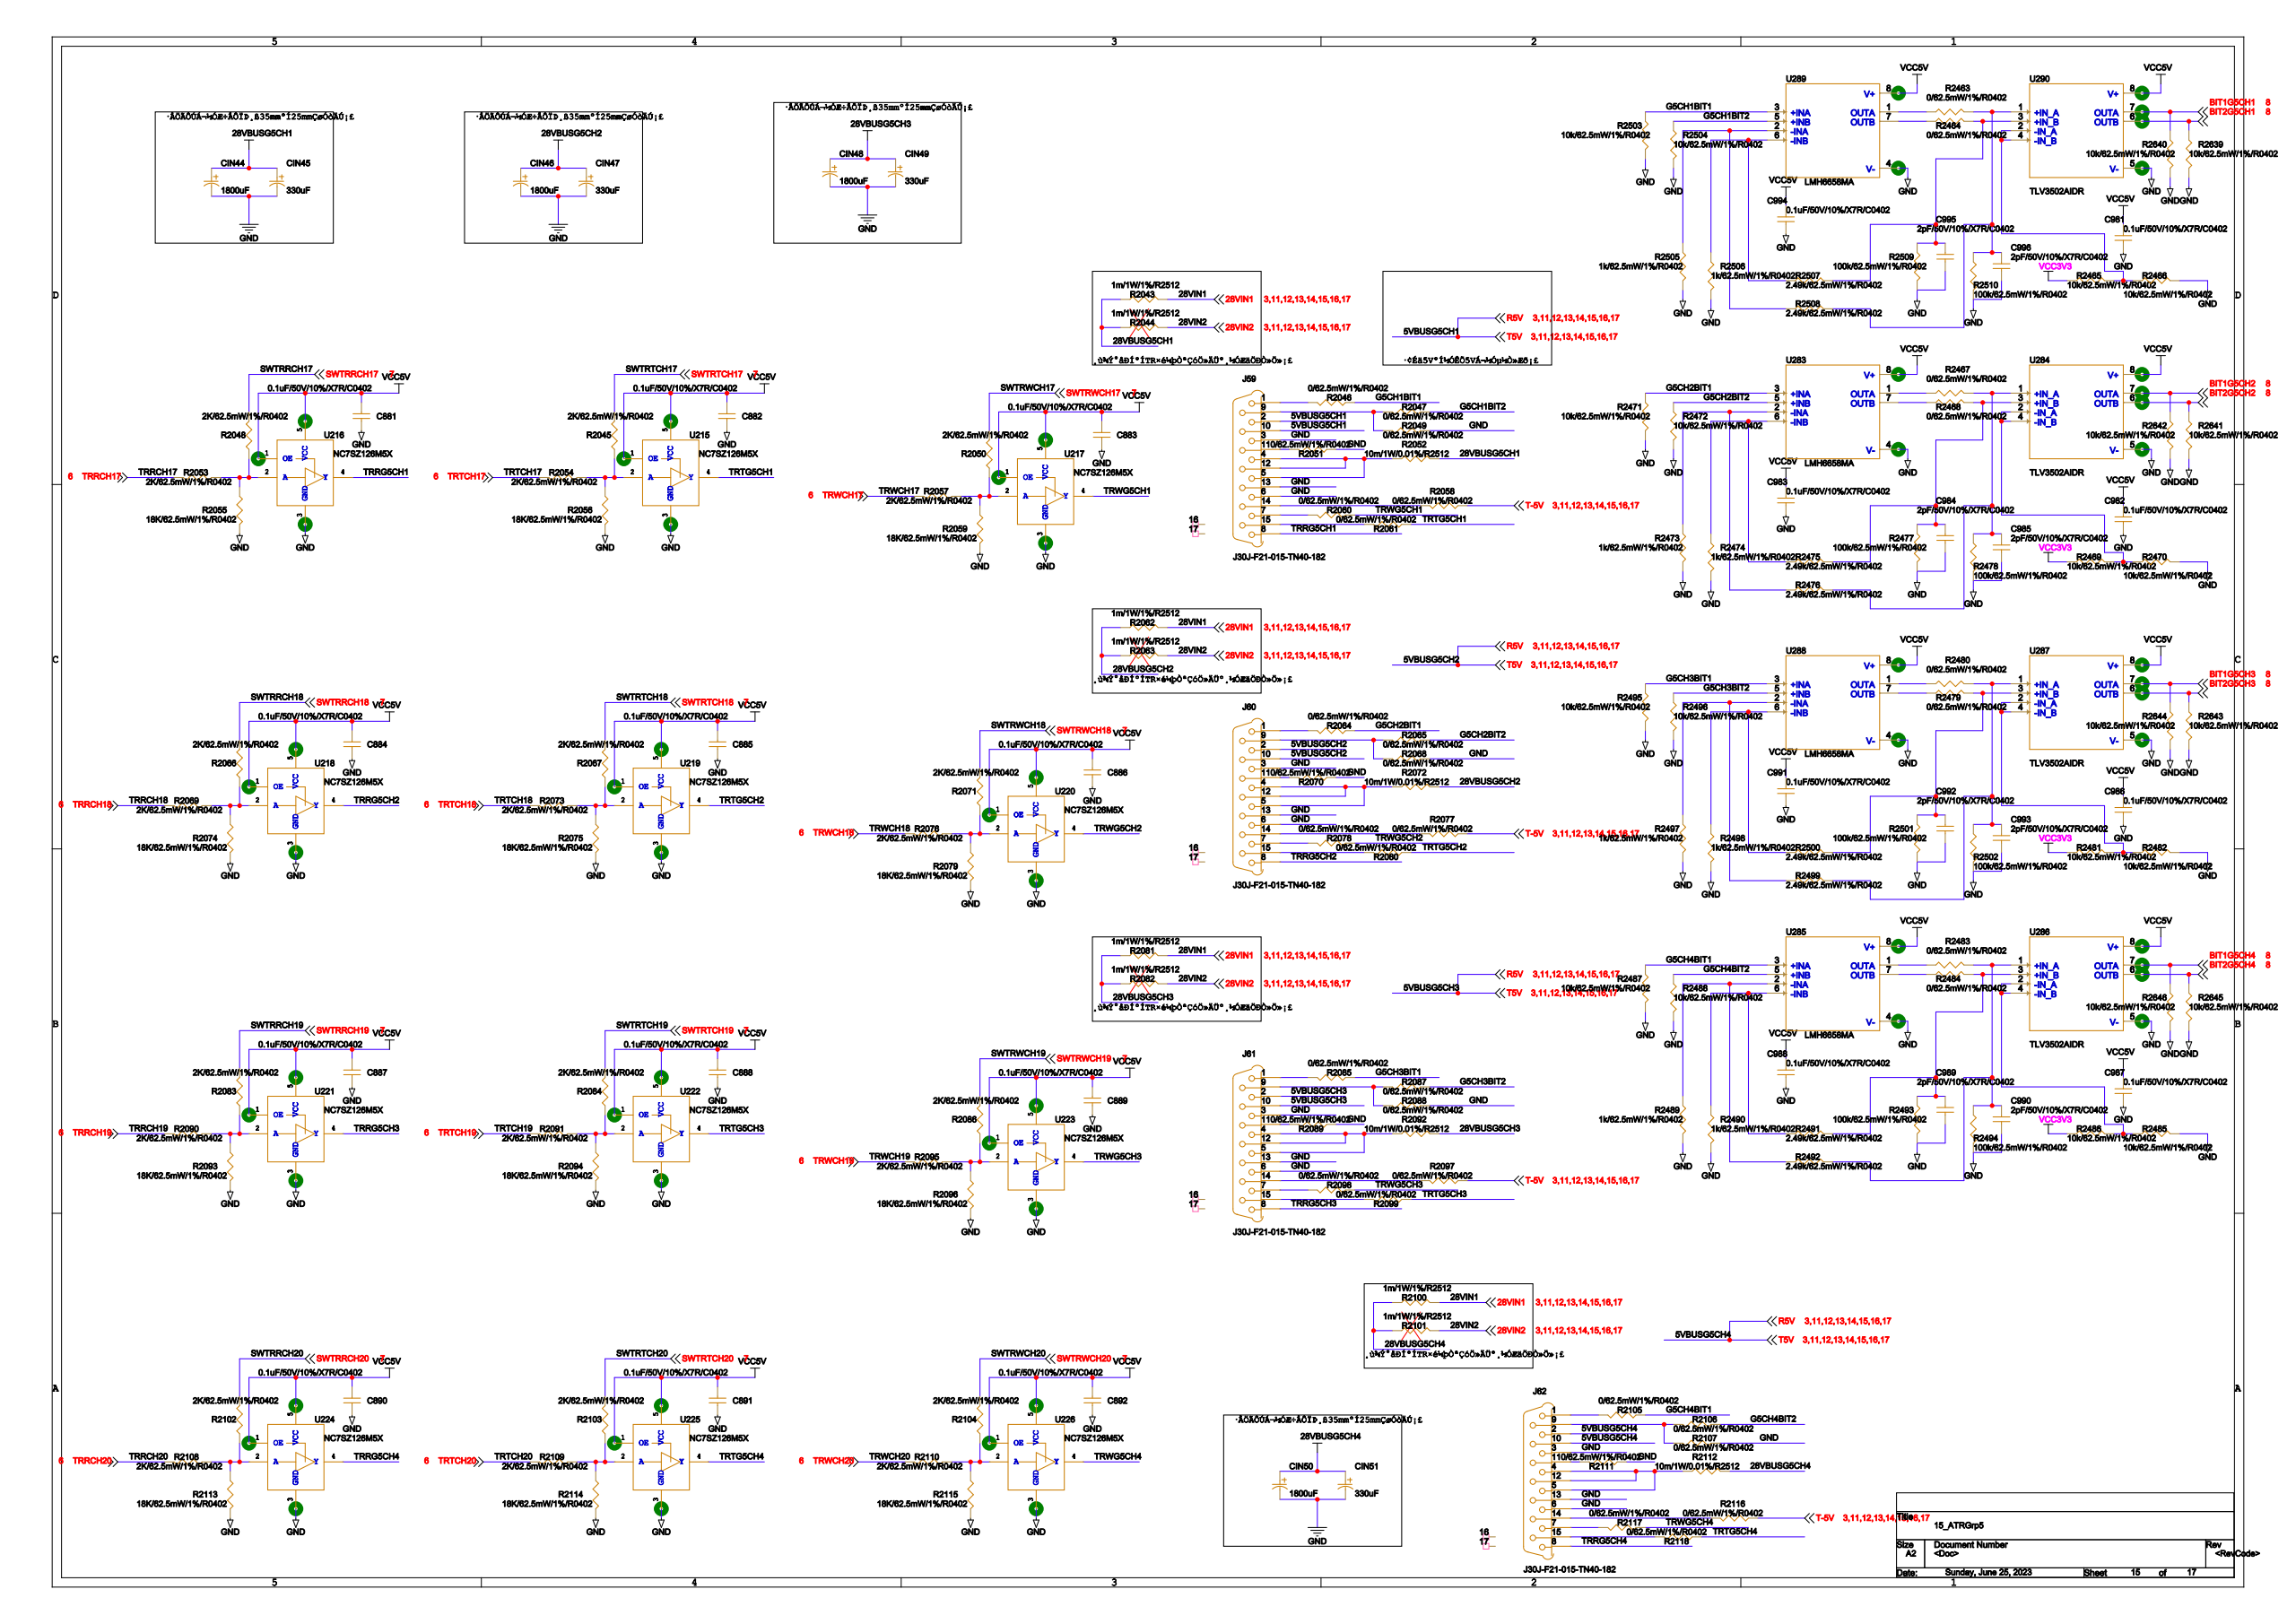Circuit board | Cadence Allegro | 2002 parts | 1538 nets | one sheet of the schematic
Parts on this sheet (reference | value | footprint):
C881 | 0.1uF/50V/10%/X7R/C0402 | 0402
C882 | 0.1uF/50V/10%/X7R/C0402 | 0402
C883 | 0.1uF/50V/10%/X7R/C0402 | 0402
C884 | 0.1uF/50V/10%/X7R/C0402 | 0402
C885 | 0.1uF/50V/10%/X7R/C0402 | 0402
C886 | 0.1uF/50V/10%/X7R/C0402 | 0402
C887 | 0.1uF/50V/10%/X7R/C0402 | 0402
C888 | 0.1uF/50V/10%/X7R/C0402 | 0402
C889 | 0.1uF/50V/10%/X7R/C0402 | 0402
C890 | 0.1uF/50V/10%/X7R/C0402 | 0402
C891 | 0.1uF/50V/10%/X7R/C0402 | 0402
C892 | 0.1uF/50V/10%/X7R/C0402 | 0402
C981 | 0.1uF/50V/10%/X7R/C0402 | 0402
C982 | 0.1uF/50V/10%/X7R/C0402 | 0402
C984 | 2pF/50V/10%/X7R/C0402 | 0402
C985 | 2pF/50V/10%/X7R/C0402 | 0402
C986 | 0.1uF/50V/10%/X7R/C0402 | 0402
C987 | 0.1uF/50V/10%/X7R/C0402 | 0402
C989 | 2pF/50V/10%/X7R/C0402 | 0402
C990 | 2pF/50V/10%/X7R/C0402 | 0402
C992 | 2pF/50V/10%/X7R/C0402 | 0402
C993 | 2pF/50V/10%/X7R/C0402 | 0402
C995 | 2pF/50V/10%/X7R/C0402 | 0402
C996 | 2pF/50V/10%/X7R/C0402 | 0402
CIN44 | ECF1HM182M27OTPO | AP-SMD_BD18-L27-W6_6-LS7_21
CIN45 | ECF1JM331G20OTPO | AP-SMD_BD10-L20-W6_6-LS7_21
CIN46 | ECF1HM182M27OTPO | AP-SMD_BD18-L27-W6_6-LS7_21
CIN47 | ECF1JM331G20OTPO | AP-SMD_BD10-L20-W6_6-LS7_21
CIN48 | ECF1HM182M27OTPO | AP-SMD_BD18-L27-W6_6-LS7_21
CIN49 | ECF1JM331G20OTPO | AP-SMD_BD10-L20-W6_6-LS7_21
CIN50 | ECF1HM182M27OTPO | AP-SMD_BD18-L27-W6_6-LS7_21
CIN51 | ECF1JM331G20OTPO | AP-SMD_BD10-L20-W6_6-LS7_21
J59 | J30J-F21-015-TN40-182 | J30J-F21-015-TN40-182
J60 | J30J-F21-015-TN40-182 | J30J-F21-015-TN40-182
J61 | J30J-F21-015-TN40-182 | J30J-F21-015-TN40-182
J62 | J30J-F21-015-TN40-182 | J30J-F21-015-TN40-182
R2043 | 1m/1W/1%/R2512 | 2512
R2044 | 1m/1W/1%/R2512 | 2512
R2045 | 2K/62.5mW/1%/R0402 | 0402
R2046 | 0/62.5mW/1%/R0402 | 0402
R2047 | 0/62.5mW/1%/R0402 | 0402
R2048 | 2K/62.5mW/1%/R0402 | 0402
R2049 | 0/62.5mW/1%/R0402 | 0402
R2050 | 2K/62.5mW/1%/R0402 | 0402
R2051 | 0/62.5mW/1%/R0402 | 0402
R2052 | 10m/1W/0.01%/R2512 | 2512
R2053 | 2K/62.5mW/1%/R0402 | 0402
R2054 | 2K/62.5mW/1%/R0402 | 0402
R2055 | 18K/62.5mW/1%/R0402 | 0402
R2056 | 18K/62.5mW/1%/R0402 | 0402
R2057 | 2K/62.5mW/1%/R0402 | 0402
R2058 | 0/62.5mW/1%/R0402 | 0402
R2059 | 18K/62.5mW/1%/R0402 | 0402
R2060 | 0/62.5mW/1%/R0402 | 0402
R2061 | 0/62.5mW/1%/R0402 | 0402
R2062 | 1m/1W/1%/R2512 | 2512
R2063 | 1m/1W/1%/R2512 | 2512
R2064 | 0/62.5mW/1%/R0402 | 0402
R2065 | 0/62.5mW/1%/R0402 | 0402
R2066 | 2K/62.5mW/1%/R0402 | 0402
R2067 | 2K/62.5mW/1%/R0402 | 0402
R2068 | 0/62.5mW/1%/R0402 | 0402
R2069 | 2K/62.5mW/1%/R0402 | 0402
R2070 | 0/62.5mW/1%/R0402 | 0402
R2071 | 2K/62.5mW/1%/R0402 | 0402
R2072 | 10m/1W/0.01%/R2512 | 2512
R2073 | 2K/62.5mW/1%/R0402 | 0402
R2074 | 18K/62.5mW/1%/R0402 | 0402
R2075 | 18K/62.5mW/1%/R0402 | 0402
R2076 | 2K/62.5mW/1%/R0402 | 0402
R2077 | 0/62.5mW/1%/R0402 | 0402
R2078 | 0/62.5mW/1%/R0402 | 0402
R2079 | 18K/62.5mW/1%/R0402 | 0402
R2080 | 0/62.5mW/1%/R0402 | 0402
R2081 | 1m/1W/1%/R2512 | 2512
R2082 | 1m/1W/1%/R2512 | 2512
R2083 | 2K/62.5mW/1%/R0402 | 0402
R2084 | 2K/62.5mW/1%/R0402 | 0402
R2085 | 0/62.5mW/1%/R0402 | 0402
R2086 | 2K/62.5mW/1%/R0402 | 0402
R2087 | 0/62.5mW/1%/R0402 | 0402
R2088 | 0/62.5mW/1%/R0402 | 0402
R2089 | 0/62.5mW/1%/R0402 | 0402
R2090 | 2K/62.5mW/1%/R0402 | 0402
R2091 | 2K/62.5mW/1%/R0402 | 0402
R2092 | 10m/1W/0.01%/R2512 | 2512
R2093 | 18K/62.5mW/1%/R0402 | 0402
R2094 | 18K/62.5mW/1%/R0402 | 0402
R2095 | 2K/62.5mW/1%/R0402 | 0402
R2096 | 18K/62.5mW/1%/R0402 | 0402
R2097 | 0/62.5mW/1%/R0402 | 0402
R2098 | 0/62.5mW/1%/R0402 | 0402
R2099 | 0/62.5mW/1%/R0402 | 0402
R2100 | 1m/1W/1%/R2512 | 2512
R2101 | 1m/1W/1%/R2512 | 2512
R2102 | 2K/62.5mW/1%/R0402 | 0402
R2103 | 2K/62.5mW/1%/R0402 | 0402
R2104 | 2K/62.5mW/1%/R0402 | 0402
R2105 | 0/62.5mW/1%/R0402 | 0402
R2106 | 0/62.5mW/1%/R0402 | 0402
R2107 | 0/62.5mW/1%/R0402 | 0402
R2108 | 2K/62.5mW/1%/R0402 | 0402
R2109 | 2K/62.5mW/1%/R0402 | 0402
R2110 | 2K/62.5mW/1%/R0402 | 0402
R2111 | 0/62.5mW/1%/R0402 | 0402
R2112 | 10m/1W/0.01%/R2512 | 2512
R2113 | 18K/62.5mW/1%/R0402 | 0402
R2114 | 18K/62.5mW/1%/R0402 | 0402
R2115 | 18K/62.5mW/1%/R0402 | 0402
R2116 | 0/62.5mW/1%/R0402 | 0402
R2117 | 0/62.5mW/1%/R0402 | 0402
R2118 | 0/62.5mW/1%/R0402 | 0402
R2463 | 0/62.5mW/1%/R0402 | 0402
R2464 | 0/62.5mW/1%/R0402 | 0402
R2465 | 10k/62.5mW/1%/R0402 | 0402
R2466 | 10k/62.5mW/1%/R0402 | 0402
R2467 | 0/62.5mW/1%/R0402 | 0402
R2468 | 0/62.5mW/1%/R0402 | 0402
R2469 | 10k/62.5mW/1%/R0402 | 0402
R2470 | 10k/62.5mW/1%/R0402 | 0402
R2471 | 10k/62.5mW/1%/R0402 | 0402
R2472 | 10k/62.5mW/1%/R0402 | 0402
R2473 | 1K/62.5mW/1%/R0402 | 0402
R2474 | 1K/62.5mW/1%/R0402 | 0402
R2476 | 2.49k/62.5mW/1%/R0402 | 0402
R2477 | 100k/62.5mW/1%/R0402 | 0402
R2478 | 100k/62.5mW/1%/R0402 | 0402
R2479 | 0/62.5mW/1%/R0402 | 0402
R2480 | 0/62.5mW/1%/R0402 | 0402
R2481 | 10k/62.5mW/1%/R0402 | 0402
R2482 | 10k/62.5mW/1%/R0402 | 0402
R2483 | 0/62.5mW/1%/R0402 | 0402
R2484 | 0/62.5mW/1%/R0402 | 0402
R2485 | 10k/62.5mW/1%/R0402 | 0402
R2486 | 10k/62.5mW/1%/R0402 | 0402
R2487 | 10k/62.5mW/1%/R0402 | 0402
R2488 | 10k/62.5mW/1%/R0402 | 0402
R2489 | 1K/62.5mW/1%/R0402 | 0402
R2490 | 1K/62.5mW/1%/R0402 | 0402
R2492 | 2.49k/62.5mW/1%/R0402 | 0402
R2493 | 100k/62.5mW/1%/R0402 | 0402
R2494 | 100k/62.5mW/1%/R0402 | 0402
R2495 | 10k/62.5mW/1%/R0402 | 0402
R2496 | 10k/62.5mW/1%/R0402 | 0402
R2497 | 1K/62.5mW/1%/R0402 | 0402
R2498 | 1K/62.5mW/1%/R0402 | 0402
R2499 | 2.49k/62.5mW/1%/R0402 | 0402
R2500 | 2.49k/62.5mW/1%/R0402 | 0402
R2501 | 100k/62.5mW/1%/R0402 | 0402
R2502 | 100k/62.5mW/1%/R0402 | 0402
R2503 | 10k/62.5mW/1%/R0402 | 0402
R2504 | 10k/62.5mW/1%/R0402 | 0402
R2505 | 1K/62.5mW/1%/R0402 | 0402
R2506 | 1K/62.5mW/1%/R0402 | 0402
R2508 | 2.49k/62.5mW/1%/R0402 | 0402
R2509 | 100k/62.5mW/1%/R0402 | 0402
R2510 | 100k/62.5mW/1%/R0402 | 0402
R2639 | 10k/62.5mW/1%/R0402 | 0402
R2640 | 10k/62.5mW/1%/R0402 | 0402
R2641 | 10k/62.5mW/1%/R0402 | 0402
R2642 | 10k/62.5mW/1%/R0402 | 0402
R2643 | 10k/62.5mW/1%/R0402 | 0402
R2644 | 10k/62.5mW/1%/R0402 | 0402
R2645 | 10k/62.5mW/1%/R0402 | 0402
R2646 | 10k/62.5mW/1%/R0402 | 0402
U215 | NC7SZ126M5X | SOT-23-5
U216 | NC7SZ126M5X | SOT-23-5
U217 | NC7SZ126M5X | SOT-23-5
U218 | NC7SZ126M5X | SOT-23-5
U219 | NC7SZ126M5X | SOT-23-5
U220 | NC7SZ126M5X | SOT-23-5
U221 | NC7SZ126M5X | SOT-23-5
U222 | NC7SZ126M5X | SOT-23-5
U223 | NC7SZ126M5X | SOT-23-5
U224 | NC7SZ126M5X | SOT-23-5
U225 | NC7SZ126M5X | SOT-23-5
U226 | NC7SZ126M5X | SOT-23-5
U283 | LMH6658MA | SOIC127P599X175-8N
U285 | LMH6658MA | SOIC127P599X175-8N
U287 | TLV3502AIDR | SOIC127P599X175-8N
U289 | LMH6658MA | SOIC127P599X175-8N
Nets of these parts (net: part-pin ...):
3.3V: R2465-1 R2469-1 R2481-1 R2486-1
AGND: C881-2 C882-2 C883-2 C884-2 C885-2 C886-2 C887-2 C888-2 C889-2 C890-2 C891-2 C892-2 C981-2 C982-2 C984-2 C985-2 C986-2 C987-2 C989-2 C990-2 C992-2 C993-2 C995-2 C996-2 CIN44-2 CIN45-2 CIN46-2 CIN47-2 CIN48-2 CIN49-2 CIN50-2 CIN51-2 J59-3 J59-6 J59-13 J60-3 J60-6 J60-13 J61-3 J61-6 J61-13 J62-3 J62-6 J62-13 R2049-1 R2051-1 R2055-1 R2056-1 R2059-1 R2068-1 R2070-1 R2074-1 R2075-1 R2079-1 R2088-1 R2089-1 R2093-1 R2094-1 R2096-1 R2107-1 R2111-1 R2113-1 R2114-1 R2115-1 R2466-2 R2470-2 R2471-2 R2472-2 R2473-2 R2474-2 R2477-2 R2478-2 R2482-2 R2485-2 R2487-2 R2488-2 R2489-2 R2490-2 R2493-2 R2494-2 R2495-2 R2496-2 R2497-2 R2498-2 R2501-2 R2502-2 R2503-2 R2504-2 R2505-2 R2506-2 R2509-2 R2510-2 R2639-2 R2640-2 R2641-2 R2642-2 R2643-2 R2644-2 R2645-2 R2646-2 U215-3 U216-3 U217-3 U218-3 U219-3 U220-3 U221-3 U222-3 U223-3 U224-3 U225-3 U226-3 U283-4 U285-4 U287-5 U289-4
VCC5V: C881-1 C882-1 C883-1 C884-1 C885-1 C886-1 C887-1 C888-1 C889-1 C890-1 C891-1 C892-1 C981-1 C982-1 C986-1 C987-1 U215-1 U215-5 U216-1 U216-5 U217-1 U217-5 U218-1 U218-5 U219-1 U219-5 U220-1 U220-5 U221-1 U221-5 U222-1 U222-5 U223-1 U223-5 U224-1 U224-5 U225-1 U225-5 U226-1 U226-5 U283-8 U285-8 U287-8 U289-8
28VIN1: R2043-2 R2044-2 R2062-2 R2063-2 R2081-2 R2082-2 R2100-2 R2101-2
R5V: J59-2 J59-10 J60-2 J60-10 J61-2 J61-10 J62-2 J62-10
T-5V: R2058-1 R2077-1 R2097-1 R2116-1
N24406183: R2474-1 U283-6
N24406193: C984-1 R2468-2 R2477-1
N24406171: R2473-1 R2476-1 U283-2
N24406191: C985-1 R2467-2 R2476-2 R2478-1
N24406737: R2490-1 U285-6
N24406747: C989-1 R2484-2 R2493-1
N24406725: R2489-1 R2492-1 U285-2
N24406745: C990-1 R2483-2 R2492-2 R2494-1
N24406549: R2497-1 R2499-1
N24406565: C993-1 R2480-2 R2499-2 R2502-1 U287-1
N24406553: R2498-1 R2500-1
N24406567: C992-1 R2479-2 R2500-2 R2501-1 U287-3
N24406003: R2506-1 U289-6
N24406013: C995-1 R2464-2 R2509-1
N24405999: R2505-1 R2508-1 U289-2
N24406011: C996-1 R2463-2 R2508-2 R2510-1
G5CH2BIT1: R2064-1 R2471-1 U283-3
G5CH2BIT2: R2065-1 R2472-1 U283-5
N24406187: R2467-1 U283-1
N24406189: R2468-1 U283-7
G5CH4BIT1: R2105-1 R2487-1 U285-3
G5CH4BIT2: R2106-1 R2488-1 U285-5
N24406741: R2483-1 U285-1
N24406743: R2484-1 U285-7
G5CH3BIT1: R2085-1 R2495-1
G5CH3BIT2: R2087-1 R2496-1
N24406561: R2480-1
N24406563: R2479-1
G5CH1BIT1: R2046-1 R2503-1 U289-3
G5CH1BIT2: R2047-1 R2504-1 U289-5
N24406007: R2463-1 U289-1
N24406009: R2464-1 U289-7
N24406245: R2469-2 R2470-1
BIT1G5CH2: R2642-1
BIT2G5CH2: R2641-1
N24406799: R2485-1 R2486-2
BIT1G5CH4: R2646-1
BIT2G5CH4: R2645-1
N24406619: R2481-2 R2482-1 U287-2 U287-4
BIT1G5CH3: R2644-1 U287-7
BIT2G5CH3: R2643-1 U287-6
N24406065: R2465-2 R2466-1
BIT1G5CH1: R2640-1
BIT2G5CH1: R2639-1
N23730929: J59-1 R2046-2
N23730942: J59-11 R2051-2
N23730944: J59-4 J59-5 J59-12 R2052-1
N23730956: J59-14 R2058-2
N23730960: J59-15 R2061-2
N23730958: J59-7 R2060-2
TRRG5CH1: J59-8 U216-4
N23730931: J59-9 R2047-2 R2049-2
N23731488: J60-1 R2064-2
N23731501: J60-11 R2070-2
N23731503: J60-4 J60-5 J60-12 R2072-1
N23731515: J60-14 R2077-2
N23731519: J60-15 R2080-2
N23731517: J60-7 R2078-2
TRRG5CH2: J60-8 U218-4
N23731490: J60-9 R2065-2 R2068-2
N23732115: J61-1 R2085-2
N23732128: J61-11 R2089-2
N23732130: J61-4 J61-5 J61-12 R2092-1
N23732142: J61-14 R2097-2
N23732146: J61-15 R2099-2
N23732144: J61-7 R2098-2
TRRG5CH3: J61-8 U221-4
N23732117: J61-9 R2087-2 R2088-2
N23732747: J62-1 R2105-2
N23732760: J62-11 R2111-2
N23732762: J62-4 J62-5 J62-12 R2112-1
N23732774: J62-14 R2116-2
N23732778: J62-15 R2118-2
N23732776: J62-7 R2117-2
TRRG5CH4: J62-8 U224-4
N23732749: J62-9 R2106-2 R2107-2
28VBUSG5CH1: CIN44-1 CIN45-1 R2043-1 R2044-1 R2052-2
28VBUSG5CH2: CIN46-1 CIN47-1 R2062-1 R2063-1 R2072-2
28VBUSG5CH3: CIN48-1 CIN49-1 R2081-1 R2082-1 R2092-2
28VBUSG5CH4: CIN50-1 CIN51-1 R2100-1 R2101-1 R2112-2
SWTRTCH17: R2045-1
N24013764: R2045-2 R2054-2 R2056-2 U215-2
SWTRRCH17: R2048-1
N24014744: R2048-2 R2053-2 R2055-2 U216-2
SWTRWCH17: R2050-1
N24014252: R2050-2 R2057-2 R2059-2 U217-2
TRRCH17: R2053-1
TRTCH17: R2054-1
TRWCH17: R2057-1
SWTRRCH18: R2066-1
N24014862: R2066-2 R2069-2 R2074-2 U218-2
SWTRTCH18: R2067-1
N24013882: R2067-2 R2073-2 R2075-2 U219-2
TRRCH18: R2069-1
SWTRWCH18: R2071-1
N24014374: R2071-2 R2076-2 R2079-2 U220-2
TRTCH18: R2073-1
TRWCH18: R2076-1
SWTRRCH19: R2083-1
N24014988: R2083-2 R2090-2 R2093-2 U221-2
SWTRTCH19: R2084-1
N24014008: R2084-2 R2091-2 R2094-2 U222-2
SWTRWCH19: R2086-1
N24014496: R2086-2 R2095-2 R2096-2 U223-2
TRRCH19: R2090-1
TRTCH19: R2091-1
TRWCH19: R2095-1
SWTRRCH20: R2102-1
N24015106: R2102-2 R2108-2 R2113-2 U224-2
SWTRTCH20: R2103-1
N24014130: R2103-2 R2109-2 R2114-2 U225-2
SWTRWCH20: R2104-1
N24014618: R2104-2 R2110-2 R2115-2 U226-2
TRRCH20: R2108-1
TRTCH20: R2109-1
TRWCH20: R2110-1
TRTG5CH1: R2061-1 U215-4
TRWG5CH1: R2060-1 U217-4
TRTG5CH2: R2080-1 U219-4
TRWG5CH2: R2078-1 U220-4
TRTG5CH3: R2099-1 U222-4
TRWG5CH3: R2098-1 U223-4
TRTG5CH4: R2118-1 U225-4
TRWG5CH4: R2117-1 U226-4